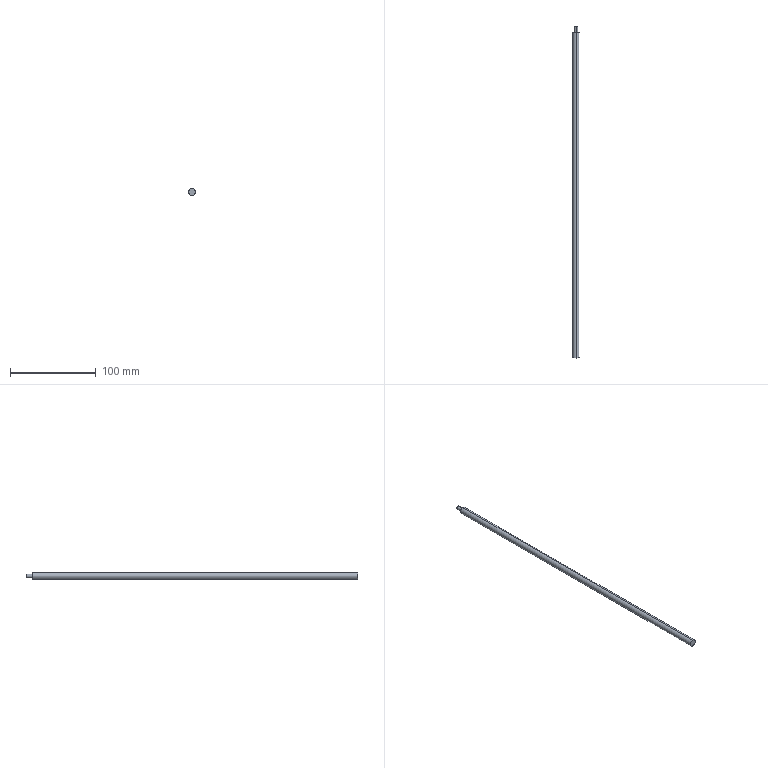Part | STEP file | Tr8 lead screw V1.201001 | 1 solid | 7 faces | box 8 x 388 x 8 mm | volume 19201 mm3 | cylinder 4 | plane 3 | commonest cylinder face diameters 4 x2 8 x2
STEP:
#1=CARTESIAN_POINT('',(0.,0.,0.));
#2=DIRECTION('',(0.,0.,1.));
#3=DIRECTION('',(1.,0.,0.));
#4=AXIS2_PLACEMENT_3D('',#1,#2,#3);
#5=CARTESIAN_POINT('',(0.,388.,2.));
#6=VERTEX_POINT('',#5);
#7=CARTESIAN_POINT('',(0.,388.,-2.));
#8=VERTEX_POINT('',#7);
#9=CARTESIAN_POINT('',(0.,388.,0.));
#10=DIRECTION('',(0.,1.,0.));
#11=DIRECTION('',(0.,0.,1.));
#12=AXIS2_PLACEMENT_3D('',#9,#10,#11);
#13=CIRCLE('',#12,2.);
#14=CARTESIAN_POINT('',(0.,388.,0.));
#15=DIRECTION('',(0.,-1.,0.));
#16=DIRECTION('',(0.,0.,-1.));
#17=AXIS2_PLACEMENT_3D('',#14,#15,#16);
#18=CYLINDRICAL_SURFACE('',#17,2.);
#19=CARTESIAN_POINT('',(3.142,0.));
#20=DIRECTION('',(-1.,0.));
#21=VECTOR('',#20,1.);
#22=LINE('',#19,#21);
#23=(GEOMETRIC_REPRESENTATION_CONTEXT(2)PARAMETRIC_REPRESENTATION_CONTEXT()REPRESENTATION_CONTEXT('',''));
#24=DEFINITIONAL_REPRESENTATION('',(#22),#23);
#25=PCURVE('',#18,#24);
#26=CARTESIAN_POINT('',(0.,388.,0.));
#27=DIRECTION('',(0.,1.,0.));
#28=DIRECTION('',(0.,0.,1.));
#29=AXIS2_PLACEMENT_3D('',#26,#27,#28);
#30=PLANE('',#29);
#31=CARTESIAN_POINT('',(0.,0.));
#32=DIRECTION('',(1.,0.));
#33=AXIS2_PLACEMENT_2D('',#31,#32);
#34=CIRCLE('',#33,2.);
#35=(GEOMETRIC_REPRESENTATION_CONTEXT(2)PARAMETRIC_REPRESENTATION_CONTEXT()REPRESENTATION_CONTEXT('',''));
#36=DEFINITIONAL_REPRESENTATION('',(#34),#35);
#37=PCURVE('',#30,#36);
#38=SURFACE_CURVE('',#13,(#25,#37),.PCURVE_S1.);
#39=EDGE_CURVE('',#6,#8,#38,.T.);
#40=ORIENTED_EDGE('',*,*,#39,.F.);
#41=CARTESIAN_POINT('',(0.,380.,2.));
#42=VERTEX_POINT('',#41);
#43=CARTESIAN_POINT('',(0.,388.,2.));
#44=DIRECTION('',(0.,-1.,0.));
#45=VECTOR('',#44,1.);
#46=LINE('',#43,#45);
#47=CARTESIAN_POINT('',(3.142,0.));
#48=DIRECTION('',(0.,1.));
#49=VECTOR('',#48,1.);
#50=LINE('',#47,#49);
#51=(GEOMETRIC_REPRESENTATION_CONTEXT(2)PARAMETRIC_REPRESENTATION_CONTEXT()REPRESENTATION_CONTEXT('',''));
#52=DEFINITIONAL_REPRESENTATION('',(#50),#51);
#53=PCURVE('',#18,#52);
#54=CARTESIAN_POINT('',(0.,388.,0.));
#55=DIRECTION('',(0.,-1.,0.));
#56=DIRECTION('',(0.,0.,-1.));
#57=AXIS2_PLACEMENT_3D('',#54,#55,#56);
#58=CYLINDRICAL_SURFACE('',#57,2.);
#59=CARTESIAN_POINT('',(3.142,0.));
#60=DIRECTION('',(0.,1.));
#61=VECTOR('',#60,1.);
#62=LINE('',#59,#61);
#63=(GEOMETRIC_REPRESENTATION_CONTEXT(2)PARAMETRIC_REPRESENTATION_CONTEXT()REPRESENTATION_CONTEXT('',''));
#64=DEFINITIONAL_REPRESENTATION('',(#62),#63);
#65=PCURVE('',#58,#64);
#66=SURFACE_CURVE('',#46,(#53,#65),.PCURVE_S1.);
#67=EDGE_CURVE('',#6,#42,#66,.T.);
#68=ORIENTED_EDGE('',*,*,#67,.T.);
#69=CARTESIAN_POINT('',(0.,380.,-2.));
#70=VERTEX_POINT('',#69);
#71=CARTESIAN_POINT('',(0.,380.,0.));
#72=DIRECTION('',(0.,1.,0.));
#73=DIRECTION('',(0.,0.,1.));
#74=AXIS2_PLACEMENT_3D('',#71,#72,#73);
#75=CIRCLE('',#74,2.);
#76=CARTESIAN_POINT('',(3.142,8.));
#77=DIRECTION('',(-1.,0.));
#78=VECTOR('',#77,1.);
#79=LINE('',#76,#78);
#80=(GEOMETRIC_REPRESENTATION_CONTEXT(2)PARAMETRIC_REPRESENTATION_CONTEXT()REPRESENTATION_CONTEXT('',''));
#81=DEFINITIONAL_REPRESENTATION('',(#79),#80);
#82=PCURVE('',#18,#81);
#83=CARTESIAN_POINT('',(0.,380.,0.));
#84=DIRECTION('',(0.,1.,0.));
#85=DIRECTION('',(0.,0.,1.));
#86=AXIS2_PLACEMENT_3D('',#83,#84,#85);
#87=PLANE('',#86);
#88=CARTESIAN_POINT('',(0.,0.));
#89=DIRECTION('',(1.,0.));
#90=AXIS2_PLACEMENT_2D('',#88,#89);
#91=CIRCLE('',#90,2.);
#92=(GEOMETRIC_REPRESENTATION_CONTEXT(2)PARAMETRIC_REPRESENTATION_CONTEXT()REPRESENTATION_CONTEXT('',''));
#93=DEFINITIONAL_REPRESENTATION('',(#91),#92);
#94=PCURVE('',#87,#93);
#95=SURFACE_CURVE('',#75,(#82,#94),.PCURVE_S1.);
#96=EDGE_CURVE('',#42,#70,#95,.T.);
#97=ORIENTED_EDGE('',*,*,#96,.T.);
#98=CARTESIAN_POINT('',(0.,388.,-2.));
#99=DIRECTION('',(0.,-1.,0.));
#100=VECTOR('',#99,1.);
#101=LINE('',#98,#100);
#102=CARTESIAN_POINT('',(0.,0.));
#103=DIRECTION('',(0.,1.));
#104=VECTOR('',#103,1.);
#105=LINE('',#102,#104);
#106=(GEOMETRIC_REPRESENTATION_CONTEXT(2)PARAMETRIC_REPRESENTATION_CONTEXT()REPRESENTATION_CONTEXT('',''));
#107=DEFINITIONAL_REPRESENTATION('',(#105),#106);
#108=PCURVE('',#18,#107);
#109=CARTESIAN_POINT('',(6.283,0.));
#110=DIRECTION('',(0.,1.));
#111=VECTOR('',#110,1.);
#112=LINE('',#109,#111);
#113=(GEOMETRIC_REPRESENTATION_CONTEXT(2)PARAMETRIC_REPRESENTATION_CONTEXT()REPRESENTATION_CONTEXT('',''));
#114=DEFINITIONAL_REPRESENTATION('',(#112),#113);
#115=PCURVE('',#58,#114);
#116=SURFACE_CURVE('',#101,(#108,#115),.PCURVE_S1.);
#117=EDGE_CURVE('',#8,#70,#116,.T.);
#118=ORIENTED_EDGE('',*,*,#117,.F.);
#119=EDGE_LOOP('',(#40,#68,#97,#118));
#120=FACE_BOUND('',#119,.T.);
#121=ADVANCED_FACE('',(#120),#18,.T.);
#122=CARTESIAN_POINT('',(0.,380.,4.));
#123=VERTEX_POINT('',#122);
#124=CARTESIAN_POINT('',(0.,380.,-4.));
#125=VERTEX_POINT('',#124);
#126=CARTESIAN_POINT('',(0.,380.,0.));
#127=DIRECTION('',(0.,1.,0.));
#128=DIRECTION('',(0.,0.,1.));
#129=AXIS2_PLACEMENT_3D('',#126,#127,#128);
#130=CIRCLE('',#129,4.);
#131=CARTESIAN_POINT('',(0.,380.,0.));
#132=DIRECTION('',(0.,-1.,0.));
#133=DIRECTION('',(0.,0.,-1.));
#134=AXIS2_PLACEMENT_3D('',#131,#132,#133);
#135=CYLINDRICAL_SURFACE('',#134,4.);
#136=CARTESIAN_POINT('',(3.142,0.));
#137=DIRECTION('',(-1.,0.));
#138=VECTOR('',#137,1.);
#139=LINE('',#136,#138);
#140=(GEOMETRIC_REPRESENTATION_CONTEXT(2)PARAMETRIC_REPRESENTATION_CONTEXT()REPRESENTATION_CONTEXT('',''));
#141=DEFINITIONAL_REPRESENTATION('',(#139),#140);
#142=PCURVE('',#135,#141);
#143=CARTESIAN_POINT('',(0.,0.));
#144=DIRECTION('',(1.,0.));
#145=AXIS2_PLACEMENT_2D('',#143,#144);
#146=CIRCLE('',#145,4.);
#147=(GEOMETRIC_REPRESENTATION_CONTEXT(2)PARAMETRIC_REPRESENTATION_CONTEXT()REPRESENTATION_CONTEXT('',''));
#148=DEFINITIONAL_REPRESENTATION('',(#146),#147);
#149=PCURVE('',#87,#148);
#150=SURFACE_CURVE('',#130,(#142,#149),.PCURVE_S1.);
#151=EDGE_CURVE('',#123,#125,#150,.T.);
#152=ORIENTED_EDGE('',*,*,#151,.F.);
#153=CARTESIAN_POINT('',(0.,0.,4.));
#154=VERTEX_POINT('',#153);
#155=CARTESIAN_POINT('',(0.,380.,4.));
#156=DIRECTION('',(0.,-1.,0.));
#157=VECTOR('',#156,1.);
#158=LINE('',#155,#157);
#159=CARTESIAN_POINT('',(3.142,0.));
#160=DIRECTION('',(0.,1.));
#161=VECTOR('',#160,1.);
#162=LINE('',#159,#161);
#163=(GEOMETRIC_REPRESENTATION_CONTEXT(2)PARAMETRIC_REPRESENTATION_CONTEXT()REPRESENTATION_CONTEXT('',''));
#164=DEFINITIONAL_REPRESENTATION('',(#162),#163);
#165=PCURVE('',#135,#164);
#166=CARTESIAN_POINT('',(0.,380.,0.));
#167=DIRECTION('',(0.,-1.,0.));
#168=DIRECTION('',(0.,0.,-1.));
#169=AXIS2_PLACEMENT_3D('',#166,#167,#168);
#170=CYLINDRICAL_SURFACE('',#169,4.);
#171=CARTESIAN_POINT('',(3.142,0.));
#172=DIRECTION('',(0.,1.));
#173=VECTOR('',#172,1.);
#174=LINE('',#171,#173);
#175=(GEOMETRIC_REPRESENTATION_CONTEXT(2)PARAMETRIC_REPRESENTATION_CONTEXT()REPRESENTATION_CONTEXT('',''));
#176=DEFINITIONAL_REPRESENTATION('',(#174),#175);
#177=PCURVE('',#170,#176);
#178=SURFACE_CURVE('',#158,(#165,#177),.PCURVE_S1.);
#179=EDGE_CURVE('',#123,#154,#178,.T.);
#180=ORIENTED_EDGE('',*,*,#179,.T.);
#181=CARTESIAN_POINT('',(0.,0.,-4.));
#182=VERTEX_POINT('',#181);
#183=CARTESIAN_POINT('',(0.,0.,0.));
#184=DIRECTION('',(0.,1.,0.));
#185=DIRECTION('',(0.,0.,1.));
#186=AXIS2_PLACEMENT_3D('',#183,#184,#185);
#187=CIRCLE('',#186,4.);
#188=CARTESIAN_POINT('',(3.142,380.));
#189=DIRECTION('',(-1.,0.));
#190=VECTOR('',#189,1.);
#191=LINE('',#188,#190);
#192=(GEOMETRIC_REPRESENTATION_CONTEXT(2)PARAMETRIC_REPRESENTATION_CONTEXT()REPRESENTATION_CONTEXT('',''));
#193=DEFINITIONAL_REPRESENTATION('',(#191),#192);
#194=PCURVE('',#135,#193);
#195=CARTESIAN_POINT('',(0.,0.,0.));
#196=DIRECTION('',(0.,1.,0.));
#197=DIRECTION('',(0.,0.,1.));
#198=AXIS2_PLACEMENT_3D('',#195,#196,#197);
#199=PLANE('',#198);
#200=CARTESIAN_POINT('',(0.,0.));
#201=DIRECTION('',(1.,0.));
#202=AXIS2_PLACEMENT_2D('',#200,#201);
#203=CIRCLE('',#202,4.);
#204=(GEOMETRIC_REPRESENTATION_CONTEXT(2)PARAMETRIC_REPRESENTATION_CONTEXT()REPRESENTATION_CONTEXT('',''));
#205=DEFINITIONAL_REPRESENTATION('',(#203),#204);
#206=PCURVE('',#199,#205);
#207=SURFACE_CURVE('',#187,(#194,#206),.PCURVE_S1.);
#208=EDGE_CURVE('',#154,#182,#207,.T.);
#209=ORIENTED_EDGE('',*,*,#208,.T.);
#210=CARTESIAN_POINT('',(0.,380.,-4.));
#211=DIRECTION('',(0.,-1.,0.));
#212=VECTOR('',#211,1.);
#213=LINE('',#210,#212);
#214=CARTESIAN_POINT('',(0.,0.));
#215=DIRECTION('',(0.,1.));
#216=VECTOR('',#215,1.);
#217=LINE('',#214,#216);
#218=(GEOMETRIC_REPRESENTATION_CONTEXT(2)PARAMETRIC_REPRESENTATION_CONTEXT()REPRESENTATION_CONTEXT('',''));
#219=DEFINITIONAL_REPRESENTATION('',(#217),#218);
#220=PCURVE('',#135,#219);
#221=CARTESIAN_POINT('',(6.283,0.));
#222=DIRECTION('',(0.,1.));
#223=VECTOR('',#222,1.);
#224=LINE('',#221,#223);
#225=(GEOMETRIC_REPRESENTATION_CONTEXT(2)PARAMETRIC_REPRESENTATION_CONTEXT()REPRESENTATION_CONTEXT('',''));
#226=DEFINITIONAL_REPRESENTATION('',(#224),#225);
#227=PCURVE('',#170,#226);
#228=SURFACE_CURVE('',#213,(#220,#227),.PCURVE_S1.);
#229=EDGE_CURVE('',#125,#182,#228,.T.);
#230=ORIENTED_EDGE('',*,*,#229,.F.);
#231=EDGE_LOOP('',(#152,#180,#209,#230));
#232=FACE_BOUND('',#231,.T.);
#233=ADVANCED_FACE('',(#232),#135,.T.);
#234=ORIENTED_EDGE('',*,*,#179,.F.);
#235=CARTESIAN_POINT('',(0.,380.,0.));
#236=DIRECTION('',(0.,1.,0.));
#237=DIRECTION('',(0.,0.,1.));
#238=AXIS2_PLACEMENT_3D('',#235,#236,#237);
#239=CIRCLE('',#238,4.);
#240=CARTESIAN_POINT('',(9.425,0.));
#241=DIRECTION('',(-1.,0.));
#242=VECTOR('',#241,1.);
#243=LINE('',#240,#242);
#244=(GEOMETRIC_REPRESENTATION_CONTEXT(2)PARAMETRIC_REPRESENTATION_CONTEXT()REPRESENTATION_CONTEXT('',''));
#245=DEFINITIONAL_REPRESENTATION('',(#243),#244);
#246=PCURVE('',#170,#245);
#247=CARTESIAN_POINT('',(0.,0.));
#248=DIRECTION('',(1.,0.));
#249=AXIS2_PLACEMENT_2D('',#247,#248);
#250=CIRCLE('',#249,4.);
#251=(GEOMETRIC_REPRESENTATION_CONTEXT(2)PARAMETRIC_REPRESENTATION_CONTEXT()REPRESENTATION_CONTEXT('',''));
#252=DEFINITIONAL_REPRESENTATION('',(#250),#251);
#253=PCURVE('',#87,#252);
#254=SURFACE_CURVE('',#239,(#246,#253),.PCURVE_S1.);
#255=EDGE_CURVE('',#125,#123,#254,.T.);
#256=ORIENTED_EDGE('',*,*,#255,.F.);
#257=ORIENTED_EDGE('',*,*,#229,.T.);
#258=CARTESIAN_POINT('',(0.,0.,0.));
#259=DIRECTION('',(0.,1.,0.));
#260=DIRECTION('',(0.,0.,1.));
#261=AXIS2_PLACEMENT_3D('',#258,#259,#260);
#262=CIRCLE('',#261,4.);
#263=CARTESIAN_POINT('',(9.425,380.));
#264=DIRECTION('',(-1.,0.));
#265=VECTOR('',#264,1.);
#266=LINE('',#263,#265);
#267=(GEOMETRIC_REPRESENTATION_CONTEXT(2)PARAMETRIC_REPRESENTATION_CONTEXT()REPRESENTATION_CONTEXT('',''));
#268=DEFINITIONAL_REPRESENTATION('',(#266),#267);
#269=PCURVE('',#170,#268);
#270=CARTESIAN_POINT('',(0.,0.));
#271=DIRECTION('',(1.,0.));
#272=AXIS2_PLACEMENT_2D('',#270,#271);
#273=CIRCLE('',#272,4.);
#274=(GEOMETRIC_REPRESENTATION_CONTEXT(2)PARAMETRIC_REPRESENTATION_CONTEXT()REPRESENTATION_CONTEXT('',''));
#275=DEFINITIONAL_REPRESENTATION('',(#273),#274);
#276=PCURVE('',#199,#275);
#277=SURFACE_CURVE('',#262,(#269,#276),.PCURVE_S1.);
#278=EDGE_CURVE('',#182,#154,#277,.T.);
#279=ORIENTED_EDGE('',*,*,#278,.T.);
#280=EDGE_LOOP('',(#234,#256,#257,#279));
#281=FACE_BOUND('',#280,.T.);
#282=ADVANCED_FACE('',(#281),#170,.T.);
#283=CARTESIAN_POINT('',(0.,380.,0.));
#284=DIRECTION('',(0.,1.,0.));
#285=DIRECTION('',(0.,0.,1.));
#286=AXIS2_PLACEMENT_3D('',#283,#284,#285);
#287=CIRCLE('',#286,2.);
#288=CARTESIAN_POINT('',(0.,0.));
#289=DIRECTION('',(1.,0.));
#290=AXIS2_PLACEMENT_2D('',#288,#289);
#291=CIRCLE('',#290,2.);
#292=(GEOMETRIC_REPRESENTATION_CONTEXT(2)PARAMETRIC_REPRESENTATION_CONTEXT()REPRESENTATION_CONTEXT('',''));
#293=DEFINITIONAL_REPRESENTATION('',(#291),#292);
#294=PCURVE('',#87,#293);
#295=CARTESIAN_POINT('',(9.425,8.));
#296=DIRECTION('',(-1.,0.));
#297=VECTOR('',#296,1.);
#298=LINE('',#295,#297);
#299=(GEOMETRIC_REPRESENTATION_CONTEXT(2)PARAMETRIC_REPRESENTATION_CONTEXT()REPRESENTATION_CONTEXT('',''));
#300=DEFINITIONAL_REPRESENTATION('',(#298),#299);
#301=PCURVE('',#58,#300);
#302=SURFACE_CURVE('',#287,(#294,#301),.PCURVE_S1.);
#303=EDGE_CURVE('',#70,#42,#302,.T.);
#304=ORIENTED_EDGE('',*,*,#303,.F.);
#305=ORIENTED_EDGE('',*,*,#96,.F.);
#306=EDGE_LOOP('',(#304,#305));
#307=FACE_BOUND('',#306,.T.);
#308=ORIENTED_EDGE('',*,*,#255,.T.);
#309=ORIENTED_EDGE('',*,*,#151,.T.);
#310=EDGE_LOOP('',(#308,#309));
#311=FACE_BOUND('',#310,.T.);
#312=ADVANCED_FACE('',(#307,#311),#87,.T.);
#313=ORIENTED_EDGE('',*,*,#278,.F.);
#314=ORIENTED_EDGE('',*,*,#208,.F.);
#315=EDGE_LOOP('',(#313,#314));
#316=FACE_BOUND('',#315,.T.);
#317=ADVANCED_FACE('',(#316),#199,.F.);
#318=ORIENTED_EDGE('',*,*,#67,.F.);
#319=CARTESIAN_POINT('',(0.,388.,0.));
#320=DIRECTION('',(0.,1.,0.));
#321=DIRECTION('',(0.,0.,1.));
#322=AXIS2_PLACEMENT_3D('',#319,#320,#321);
#323=CIRCLE('',#322,2.);
#324=CARTESIAN_POINT('',(9.425,0.));
#325=DIRECTION('',(-1.,0.));
#326=VECTOR('',#325,1.);
#327=LINE('',#324,#326);
#328=(GEOMETRIC_REPRESENTATION_CONTEXT(2)PARAMETRIC_REPRESENTATION_CONTEXT()REPRESENTATION_CONTEXT('',''));
#329=DEFINITIONAL_REPRESENTATION('',(#327),#328);
#330=PCURVE('',#58,#329);
#331=CARTESIAN_POINT('',(0.,0.));
#332=DIRECTION('',(1.,0.));
#333=AXIS2_PLACEMENT_2D('',#331,#332);
#334=CIRCLE('',#333,2.);
#335=(GEOMETRIC_REPRESENTATION_CONTEXT(2)PARAMETRIC_REPRESENTATION_CONTEXT()REPRESENTATION_CONTEXT('',''));
#336=DEFINITIONAL_REPRESENTATION('',(#334),#335);
#337=PCURVE('',#30,#336);
#338=SURFACE_CURVE('',#323,(#330,#337),.PCURVE_S1.);
#339=EDGE_CURVE('',#8,#6,#338,.T.);
#340=ORIENTED_EDGE('',*,*,#339,.F.);
#341=ORIENTED_EDGE('',*,*,#117,.T.);
#342=ORIENTED_EDGE('',*,*,#303,.T.);
#343=EDGE_LOOP('',(#318,#340,#341,#342));
#344=FACE_BOUND('',#343,.T.);
#345=ADVANCED_FACE('',(#344),#58,.T.);
#346=ORIENTED_EDGE('',*,*,#339,.T.);
#347=ORIENTED_EDGE('',*,*,#39,.T.);
#348=EDGE_LOOP('',(#346,#347));
#349=FACE_BOUND('',#348,.T.);
#350=ADVANCED_FACE('',(#349),#30,.T.);
#351=CLOSED_SHELL('',(#121,#233,#282,#312,#317,#345,#350));
#352=MANIFOLD_SOLID_BREP('',#351);
#353=(LENGTH_UNIT()NAMED_UNIT(*)SI_UNIT(.MILLI.,.METRE.));
#354=UNCERTAINTY_MEASURE_WITH_UNIT(LENGTH_MEASURE(0.0000001),#353,'','');
#355=(NAMED_UNIT(*)PLANE_ANGLE_UNIT()SI_UNIT($,.RADIAN.));
#356=(NAMED_UNIT(*)SI_UNIT($,.STERADIAN.)SOLID_ANGLE_UNIT());
#357=(GEOMETRIC_REPRESENTATION_CONTEXT(3)GLOBAL_UNCERTAINTY_ASSIGNED_CONTEXT((#354))GLOBAL_UNIT_ASSIGNED_CONTEXT((#353,#355,#356))REPRESENTATION_CONTEXT('',''));
#358=ADVANCED_BREP_SHAPE_REPRESENTATION('',(#4,#352),#357);